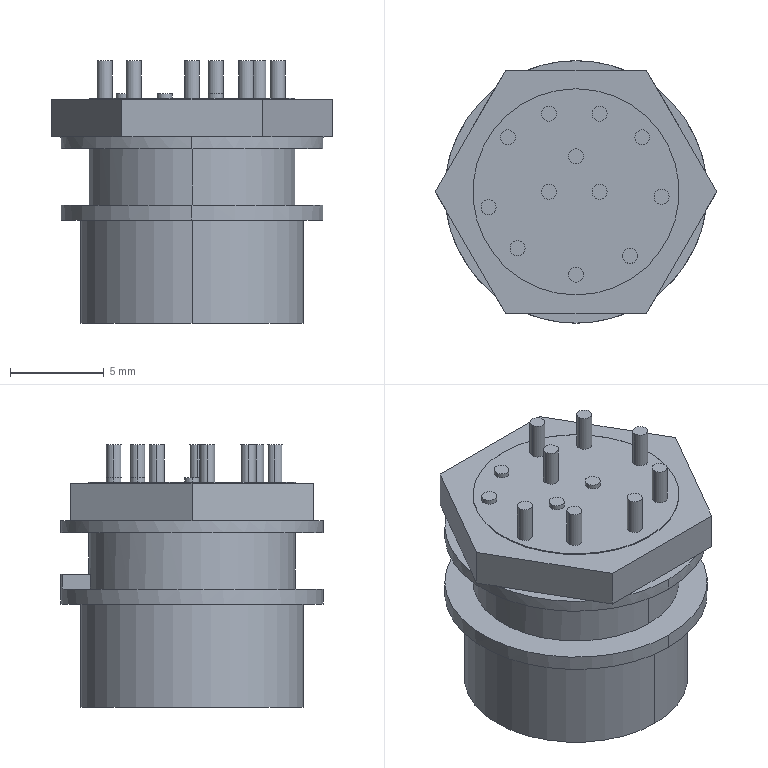Part | STEP file | ASND-0110-4216107480_SPEC | 1 solid | 82 faces | box 15.011 x 14 x 14 mm | volume 1337 mm3 | plane 42 | cylinder 40 | commonest cylinder face diameters 0.8 x24 11 x4 14 x4 6 x2 8 x2 11.3 x2